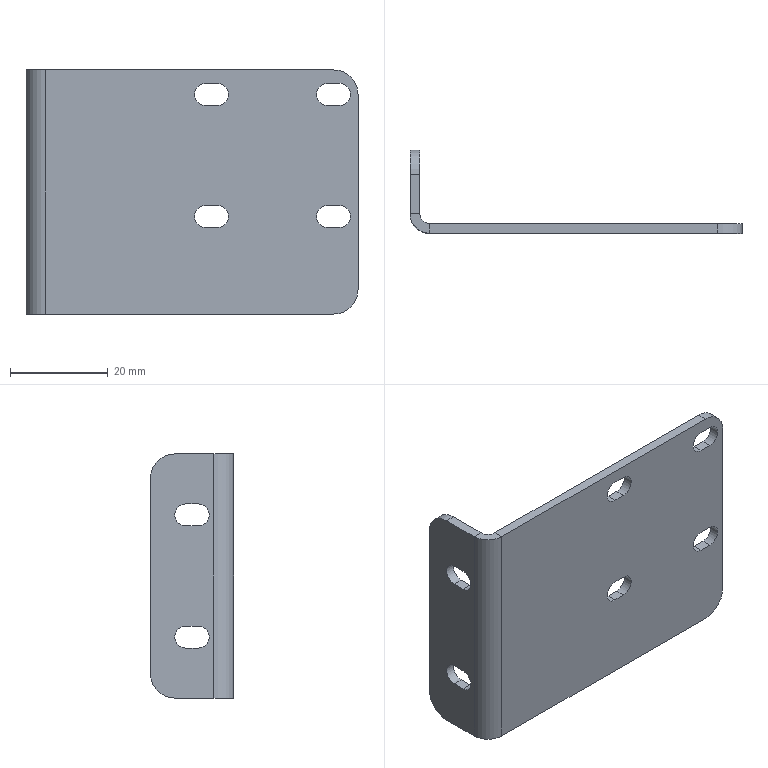Part | SolidWorks | features HoleWzd 2, Fillet 1, FlatPattern 1, SMBaseFlange 1, SheetMetal 1 | 1 solid | 42 faces | box 68 x 17 x 50 mm | volume 7802 mm3 | plane 24 | cylinder 18 | commonest cylinder face diameters 4.5 x12 10 x4 4 x1 8 x1
STEP:
#1=CARTESIAN_POINT('',(2.,-9.75,39.75));
#2=VERTEX_POINT('',#1);
#3=CARTESIAN_POINT('',(2.,-9.75,35.25));
#4=VERTEX_POINT('',#3);
#5=CARTESIAN_POINT('',(2.,-9.75,37.5));
#6=DIRECTION('',(1.,0.,0.));
#7=DIRECTION('',(0.,0.,-1.));
#8=AXIS2_PLACEMENT_3D('',#5,#6,#7);
#9=CIRCLE('',#8,2.25);
#10=EDGE_CURVE('',#2,#4,#9,.T.);
#11=ORIENTED_EDGE('',*,*,#10,.F.);
#12=CARTESIAN_POINT('',(2.,-7.25,39.75));
#13=VERTEX_POINT('',#12);
#14=CARTESIAN_POINT('',(2.,-9.75,39.75));
#15=DIRECTION('',(0.,1.,0.));
#16=VECTOR('',#15,1000.);
#17=LINE('',#14,#16);
#18=EDGE_CURVE('',#2,#13,#17,.T.);
#19=ORIENTED_EDGE('',*,*,#18,.T.);
#20=CARTESIAN_POINT('',(2.,-7.25,35.25));
#21=VERTEX_POINT('',#20);
#22=CARTESIAN_POINT('',(2.,-7.25,37.5));
#23=DIRECTION('',(1.,0.,0.));
#24=DIRECTION('',(0.,0.,-1.));
#25=AXIS2_PLACEMENT_3D('',#22,#23,#24);
#26=CIRCLE('',#25,2.25);
#27=EDGE_CURVE('',#21,#13,#26,.T.);
#28=ORIENTED_EDGE('',*,*,#27,.F.);
#29=CARTESIAN_POINT('',(2.,-9.75,35.25));
#30=DIRECTION('',(0.,1.,0.));
#31=VECTOR('',#30,1000.);
#32=LINE('',#29,#31);
#33=EDGE_CURVE('',#4,#21,#32,.T.);
#34=ORIENTED_EDGE('',*,*,#33,.F.);
#35=EDGE_LOOP('',(#11,#19,#28,#34));
#36=FACE_BOUND('',#35,.T.);
#37=CARTESIAN_POINT('',(2.,0.,45.));
#38=VERTEX_POINT('',#37);
#39=CARTESIAN_POINT('',(2.,0.,5.));
#40=VERTEX_POINT('',#39);
#41=CARTESIAN_POINT('',(2.,0.,50.));
#42=DIRECTION('',(0.,0.,-1.));
#43=VECTOR('',#42,1000.);
#44=LINE('',#41,#43);
#45=EDGE_CURVE('',#38,#40,#44,.T.);
#46=ORIENTED_EDGE('',*,*,#45,.F.);
#47=CARTESIAN_POINT('',(2.,-5.,50.));
#48=VERTEX_POINT('',#47);
#49=CARTESIAN_POINT('',(2.,-5.,45.));
#50=DIRECTION('',(1.,0.,0.));
#51=DIRECTION('',(0.,1.,0.));
#52=AXIS2_PLACEMENT_3D('',#49,#50,#51);
#53=CIRCLE('',#52,5.);
#54=EDGE_CURVE('',#38,#48,#53,.T.);
#55=ORIENTED_EDGE('',*,*,#54,.T.);
#56=CARTESIAN_POINT('',(2.,-13.,50.));
#57=VERTEX_POINT('',#56);
#58=CARTESIAN_POINT('',(2.,0.,50.));
#59=DIRECTION('',(0.,-1.,0.));
#60=VECTOR('',#59,1000.);
#61=LINE('',#58,#60);
#62=EDGE_CURVE('',#48,#57,#61,.T.);
#63=ORIENTED_EDGE('',*,*,#62,.T.);
#64=CARTESIAN_POINT('',(2.,-13.,0.));
#65=VERTEX_POINT('',#64);
#66=CARTESIAN_POINT('',(2.,-13.,50.));
#67=DIRECTION('',(0.,0.,-1.));
#68=VECTOR('',#67,1000.);
#69=LINE('',#66,#68);
#70=EDGE_CURVE('',#57,#65,#69,.T.);
#71=ORIENTED_EDGE('',*,*,#70,.T.);
#72=CARTESIAN_POINT('',(2.,-5.,0.));
#73=VERTEX_POINT('',#72);
#74=CARTESIAN_POINT('',(2.,0.,0.));
#75=DIRECTION('',(0.,-1.,0.));
#76=VECTOR('',#75,1000.);
#77=LINE('',#74,#76);
#78=EDGE_CURVE('',#73,#65,#77,.T.);
#79=ORIENTED_EDGE('',*,*,#78,.F.);
#80=CARTESIAN_POINT('',(2.,-5.,5.));
#81=DIRECTION('',(1.,0.,0.));
#82=DIRECTION('',(0.,1.,0.));
#83=AXIS2_PLACEMENT_3D('',#80,#81,#82);
#84=CIRCLE('',#83,5.);
#85=EDGE_CURVE('',#73,#40,#84,.T.);
#86=ORIENTED_EDGE('',*,*,#85,.T.);
#87=EDGE_LOOP('',(#46,#55,#63,#71,#79,#86));
#88=FACE_OUTER_BOUND('',#87,.T.);
#89=CARTESIAN_POINT('',(2.,-9.75,14.75));
#90=VERTEX_POINT('',#89);
#91=CARTESIAN_POINT('',(2.,-9.75,10.25));
#92=VERTEX_POINT('',#91);
#93=CARTESIAN_POINT('',(2.,-9.75,12.5));
#94=DIRECTION('',(1.,0.,0.));
#95=DIRECTION('',(0.,0.,-1.));
#96=AXIS2_PLACEMENT_3D('',#93,#94,#95);
#97=CIRCLE('',#96,2.25);
#98=EDGE_CURVE('',#90,#92,#97,.T.);
#99=ORIENTED_EDGE('',*,*,#98,.F.);
#100=CARTESIAN_POINT('',(2.,-7.25,14.75));
#101=VERTEX_POINT('',#100);
#102=CARTESIAN_POINT('',(2.,-9.75,14.75));
#103=DIRECTION('',(0.,1.,0.));
#104=VECTOR('',#103,1000.);
#105=LINE('',#102,#104);
#106=EDGE_CURVE('',#90,#101,#105,.T.);
#107=ORIENTED_EDGE('',*,*,#106,.T.);
#108=CARTESIAN_POINT('',(2.,-7.25,10.25));
#109=VERTEX_POINT('',#108);
#110=CARTESIAN_POINT('',(2.,-7.25,12.5));
#111=DIRECTION('',(1.,0.,0.));
#112=DIRECTION('',(0.,0.,-1.));
#113=AXIS2_PLACEMENT_3D('',#110,#111,#112);
#114=CIRCLE('',#113,2.25);
#115=EDGE_CURVE('',#109,#101,#114,.T.);
#116=ORIENTED_EDGE('',*,*,#115,.F.);
#117=CARTESIAN_POINT('',(2.,-9.75,10.25));
#118=DIRECTION('',(0.,1.,0.));
#119=VECTOR('',#118,1000.);
#120=LINE('',#117,#119);
#121=EDGE_CURVE('',#92,#109,#120,.T.);
#122=ORIENTED_EDGE('',*,*,#121,.F.);
#123=EDGE_LOOP('',(#99,#107,#116,#122));
#124=FACE_BOUND('',#123,.T.);
#125=CARTESIAN_POINT('',(2.,0.,50.));
#126=DIRECTION('',(1.,0.,0.));
#127=DIRECTION('',(0.,1.,0.));
#128=AXIS2_PLACEMENT_3D('',#125,#126,#127);
#129=PLANE('',#128);
#130=ADVANCED_FACE('',(#36,#88,#124),#129,.T.);
#131=CARTESIAN_POINT('',(61.75,-15.,47.25));
#132=VERTEX_POINT('',#131);
#133=CARTESIAN_POINT('',(64.25,-15.,47.25));
#134=VERTEX_POINT('',#133);
#135=CARTESIAN_POINT('',(61.75,-15.,47.25));
#136=DIRECTION('',(1.,0.,0.));
#137=VECTOR('',#136,1000.);
#138=LINE('',#135,#137);
#139=EDGE_CURVE('',#132,#134,#138,.T.);
#140=ORIENTED_EDGE('',*,*,#139,.F.);
#141=CARTESIAN_POINT('',(61.75,-15.,42.75));
#142=VERTEX_POINT('',#141);
#143=CARTESIAN_POINT('',(61.75,-15.,45.));
#144=DIRECTION('',(0.,1.,0.));
#145=DIRECTION('',(0.,0.,1.));
#146=AXIS2_PLACEMENT_3D('',#143,#144,#145);
#147=CIRCLE('',#146,2.25);
#148=EDGE_CURVE('',#142,#132,#147,.T.);
#149=ORIENTED_EDGE('',*,*,#148,.F.);
#150=CARTESIAN_POINT('',(64.25,-15.,42.75));
#151=VERTEX_POINT('',#150);
#152=CARTESIAN_POINT('',(61.75,-15.,42.75));
#153=DIRECTION('',(1.,0.,0.));
#154=VECTOR('',#153,1000.);
#155=LINE('',#152,#154);
#156=EDGE_CURVE('',#142,#151,#155,.T.);
#157=ORIENTED_EDGE('',*,*,#156,.T.);
#158=CARTESIAN_POINT('',(64.25,-15.,45.));
#159=DIRECTION('',(0.,1.,0.));
#160=DIRECTION('',(0.,0.,1.));
#161=AXIS2_PLACEMENT_3D('',#158,#159,#160);
#162=CIRCLE('',#161,2.25);
#163=EDGE_CURVE('',#134,#151,#162,.T.);
#164=ORIENTED_EDGE('',*,*,#163,.F.);
#165=EDGE_LOOP('',(#140,#149,#157,#164));
#166=FACE_BOUND('',#165,.T.);
#167=CARTESIAN_POINT('',(36.75,-15.,42.75));
#168=VERTEX_POINT('',#167);
#169=CARTESIAN_POINT('',(39.25,-15.,42.75));
#170=VERTEX_POINT('',#169);
#171=CARTESIAN_POINT('',(36.75,-15.,42.75));
#172=DIRECTION('',(1.,0.,0.));
#173=VECTOR('',#172,1000.);
#174=LINE('',#171,#173);
#175=EDGE_CURVE('',#168,#170,#174,.T.);
#176=ORIENTED_EDGE('',*,*,#175,.T.);
#177=CARTESIAN_POINT('',(39.25,-15.,47.25));
#178=VERTEX_POINT('',#177);
#179=CARTESIAN_POINT('',(39.25,-15.,45.));
#180=DIRECTION('',(0.,1.,0.));
#181=DIRECTION('',(0.,0.,1.));
#182=AXIS2_PLACEMENT_3D('',#179,#180,#181);
#183=CIRCLE('',#182,2.25);
#184=EDGE_CURVE('',#178,#170,#183,.T.);
#185=ORIENTED_EDGE('',*,*,#184,.F.);
#186=CARTESIAN_POINT('',(36.75,-15.,47.25));
#187=VERTEX_POINT('',#186);
#188=CARTESIAN_POINT('',(36.75,-15.,47.25));
#189=DIRECTION('',(1.,0.,0.));
#190=VECTOR('',#189,1000.);
#191=LINE('',#188,#190);
#192=EDGE_CURVE('',#187,#178,#191,.T.);
#193=ORIENTED_EDGE('',*,*,#192,.F.);
#194=CARTESIAN_POINT('',(36.75,-15.,45.));
#195=DIRECTION('',(0.,1.,0.));
#196=DIRECTION('',(0.,0.,1.));
#197=AXIS2_PLACEMENT_3D('',#194,#195,#196);
#198=CIRCLE('',#197,2.25);
#199=EDGE_CURVE('',#168,#187,#198,.T.);
#200=ORIENTED_EDGE('',*,*,#199,.F.);
#201=EDGE_LOOP('',(#176,#185,#193,#200));
#202=FACE_BOUND('',#201,.T.);
#203=CARTESIAN_POINT('',(36.75,-15.,22.25));
#204=VERTEX_POINT('',#203);
#205=CARTESIAN_POINT('',(39.25,-15.,22.25));
#206=VERTEX_POINT('',#205);
#207=CARTESIAN_POINT('',(36.75,-15.,22.25));
#208=DIRECTION('',(1.,0.,0.));
#209=VECTOR('',#208,1000.);
#210=LINE('',#207,#209);
#211=EDGE_CURVE('',#204,#206,#210,.T.);
#212=ORIENTED_EDGE('',*,*,#211,.F.);
#213=CARTESIAN_POINT('',(36.75,-15.,17.75));
#214=VERTEX_POINT('',#213);
#215=CARTESIAN_POINT('',(36.75,-15.,20.));
#216=DIRECTION('',(0.,1.,0.));
#217=DIRECTION('',(0.,0.,1.));
#218=AXIS2_PLACEMENT_3D('',#215,#216,#217);
#219=CIRCLE('',#218,2.25);
#220=EDGE_CURVE('',#214,#204,#219,.T.);
#221=ORIENTED_EDGE('',*,*,#220,.F.);
#222=CARTESIAN_POINT('',(39.25,-15.,17.75));
#223=VERTEX_POINT('',#222);
#224=CARTESIAN_POINT('',(36.75,-15.,17.75));
#225=DIRECTION('',(1.,0.,0.));
#226=VECTOR('',#225,1000.);
#227=LINE('',#224,#226);
#228=EDGE_CURVE('',#214,#223,#227,.T.);
#229=ORIENTED_EDGE('',*,*,#228,.T.);
#230=CARTESIAN_POINT('',(39.25,-15.,20.));
#231=DIRECTION('',(0.,1.,0.));
#232=DIRECTION('',(0.,0.,1.));
#233=AXIS2_PLACEMENT_3D('',#230,#231,#232);
#234=CIRCLE('',#233,2.25);
#235=EDGE_CURVE('',#206,#223,#234,.T.);
#236=ORIENTED_EDGE('',*,*,#235,.F.);
#237=EDGE_LOOP('',(#212,#221,#229,#236));
#238=FACE_BOUND('',#237,.T.);
#239=CARTESIAN_POINT('',(4.,-15.,50.));
#240=VERTEX_POINT('',#239);
#241=CARTESIAN_POINT('',(63.,-15.,50.));
#242=VERTEX_POINT('',#241);
#243=CARTESIAN_POINT('',(0.,-15.,50.));
#244=DIRECTION('',(1.,0.,0.));
#245=VECTOR('',#244,1000.);
#246=LINE('',#243,#245);
#247=EDGE_CURVE('',#240,#242,#246,.T.);
#248=ORIENTED_EDGE('',*,*,#247,.T.);
#249=CARTESIAN_POINT('',(68.,-15.,45.));
#250=VERTEX_POINT('',#249);
#251=CARTESIAN_POINT('',(63.,-15.,45.));
#252=DIRECTION('',(0.,1.,0.));
#253=DIRECTION('',(0.,0.,1.));
#254=AXIS2_PLACEMENT_3D('',#251,#252,#253);
#255=CIRCLE('',#254,5.);
#256=EDGE_CURVE('',#242,#250,#255,.T.);
#257=ORIENTED_EDGE('',*,*,#256,.T.);
#258=CARTESIAN_POINT('',(68.,-15.,5.));
#259=VERTEX_POINT('',#258);
#260=CARTESIAN_POINT('',(68.,-15.,50.));
#261=DIRECTION('',(0.,0.,-1.));
#262=VECTOR('',#261,1000.);
#263=LINE('',#260,#262);
#264=EDGE_CURVE('',#250,#259,#263,.T.);
#265=ORIENTED_EDGE('',*,*,#264,.T.);
#266=CARTESIAN_POINT('',(63.,-15.,0.));
#267=VERTEX_POINT('',#266);
#268=CARTESIAN_POINT('',(63.,-15.,5.));
#269=DIRECTION('',(0.,1.,0.));
#270=DIRECTION('',(0.,0.,1.));
#271=AXIS2_PLACEMENT_3D('',#268,#269,#270);
#272=CIRCLE('',#271,5.);
#273=EDGE_CURVE('',#259,#267,#272,.T.);
#274=ORIENTED_EDGE('',*,*,#273,.T.);
#275=CARTESIAN_POINT('',(4.,-15.,0.));
#276=VERTEX_POINT('',#275);
#277=CARTESIAN_POINT('',(0.,-15.,0.));
#278=DIRECTION('',(1.,0.,0.));
#279=VECTOR('',#278,1000.);
#280=LINE('',#277,#279);
#281=EDGE_CURVE('',#276,#267,#280,.T.);
#282=ORIENTED_EDGE('',*,*,#281,.F.);
#283=CARTESIAN_POINT('',(4.,-15.,50.));
#284=DIRECTION('',(0.,0.,-1.));
#285=VECTOR('',#284,1000.);
#286=LINE('',#283,#285);
#287=EDGE_CURVE('',#240,#276,#286,.T.);
#288=ORIENTED_EDGE('',*,*,#287,.F.);
#289=EDGE_LOOP('',(#248,#257,#265,#274,#282,#288));
#290=FACE_OUTER_BOUND('',#289,.T.);
#291=CARTESIAN_POINT('',(61.75,-15.,17.75));
#292=VERTEX_POINT('',#291);
#293=CARTESIAN_POINT('',(61.75,-15.,22.25));
#294=VERTEX_POINT('',#293);
#295=CARTESIAN_POINT('',(61.75,-15.,20.));
#296=DIRECTION('',(0.,1.,0.));
#297=DIRECTION('',(0.,0.,1.));
#298=AXIS2_PLACEMENT_3D('',#295,#296,#297);
#299=CIRCLE('',#298,2.25);
#300=EDGE_CURVE('',#292,#294,#299,.T.);
#301=ORIENTED_EDGE('',*,*,#300,.F.);
#302=CARTESIAN_POINT('',(64.25,-15.,17.75));
#303=VERTEX_POINT('',#302);
#304=CARTESIAN_POINT('',(61.75,-15.,17.75));
#305=DIRECTION('',(1.,0.,0.));
#306=VECTOR('',#305,1000.);
#307=LINE('',#304,#306);
#308=EDGE_CURVE('',#292,#303,#307,.T.);
#309=ORIENTED_EDGE('',*,*,#308,.T.);
#310=CARTESIAN_POINT('',(64.25,-15.,22.25));
#311=VERTEX_POINT('',#310);
#312=CARTESIAN_POINT('',(64.25,-15.,20.));
#313=DIRECTION('',(0.,1.,0.));
#314=DIRECTION('',(0.,0.,1.));
#315=AXIS2_PLACEMENT_3D('',#312,#313,#314);
#316=CIRCLE('',#315,2.25);
#317=EDGE_CURVE('',#311,#303,#316,.T.);
#318=ORIENTED_EDGE('',*,*,#317,.F.);
#319=CARTESIAN_POINT('',(61.75,-15.,22.25));
#320=DIRECTION('',(1.,0.,0.));
#321=VECTOR('',#320,1000.);
#322=LINE('',#319,#321);
#323=EDGE_CURVE('',#294,#311,#322,.T.);
#324=ORIENTED_EDGE('',*,*,#323,.F.);
#325=EDGE_LOOP('',(#301,#309,#318,#324));
#326=FACE_BOUND('',#325,.T.);
#327=CARTESIAN_POINT('',(0.,-15.,50.));
#328=DIRECTION('',(0.,1.,0.));
#329=DIRECTION('',(0.,0.,1.));
#330=AXIS2_PLACEMENT_3D('',#327,#328,#329);
#331=PLANE('',#330);
#332=ADVANCED_FACE('',(#166,#202,#238,#290,#326),#331,.T.);
#333=CARTESIAN_POINT('',(0.,-13.,50.));
#334=VERTEX_POINT('',#333);
#335=CARTESIAN_POINT('',(0.,-13.,50.));
#336=DIRECTION('',(1.,0.,0.));
#337=VECTOR('',#336,1000.);
#338=LINE('',#335,#337);
#339=EDGE_CURVE('',#334,#57,#338,.T.);
#340=ORIENTED_EDGE('',*,*,#339,.F.);
#341=CARTESIAN_POINT('',(4.,-17.,50.));
#342=VERTEX_POINT('',#341);
#343=CARTESIAN_POINT('',(4.,-13.,50.));
#344=DIRECTION('',(0.,0.,1.));
#345=DIRECTION('',(-1.,0.,0.));
#346=AXIS2_PLACEMENT_3D('',#343,#344,#345);
#347=CIRCLE('',#346,4.);
#348=EDGE_CURVE('',#334,#342,#347,.T.);
#349=ORIENTED_EDGE('',*,*,#348,.T.);
#350=CARTESIAN_POINT('',(4.,-15.,50.));
#351=DIRECTION('',(0.,-1.,0.));
#352=VECTOR('',#351,1000.);
#353=LINE('',#350,#352);
#354=EDGE_CURVE('',#240,#342,#353,.T.);
#355=ORIENTED_EDGE('',*,*,#354,.F.);
#356=CARTESIAN_POINT('',(4.,-13.,50.));
#357=DIRECTION('',(0.,0.,1.));
#358=DIRECTION('',(1.,0.,0.));
#359=AXIS2_PLACEMENT_3D('',#356,#357,#358);
#360=CIRCLE('',#359,2.);
#361=EDGE_CURVE('',#57,#240,#360,.T.);
#362=ORIENTED_EDGE('',*,*,#361,.F.);
#363=EDGE_LOOP('',(#340,#349,#355,#362));
#364=FACE_OUTER_BOUND('',#363,.T.);
#365=CARTESIAN_POINT('',(0.,-13.,50.));
#366=DIRECTION('',(0.,0.,1.));
#367=DIRECTION('',(1.,0.,0.));
#368=AXIS2_PLACEMENT_3D('',#365,#366,#367);
#369=PLANE('',#368);
#370=ADVANCED_FACE('',(#364),#369,.T.);
#371=ORIENTED_EDGE('',*,*,#62,.F.);
#372=CARTESIAN_POINT('',(0.,-5.,50.));
#373=VERTEX_POINT('',#372);
#374=CARTESIAN_POINT('',(4.,-5.,50.));
#375=DIRECTION('',(-1.,0.,0.));
#376=VECTOR('',#375,1000.);
#377=LINE('',#374,#376);
#378=EDGE_CURVE('',#48,#373,#377,.T.);
#379=ORIENTED_EDGE('',*,*,#378,.T.);
#380=CARTESIAN_POINT('',(0.,0.,50.));
#381=DIRECTION('',(0.,-1.,0.));
#382=VECTOR('',#381,1000.);
#383=LINE('',#380,#382);
#384=EDGE_CURVE('',#373,#334,#383,.T.);
#385=ORIENTED_EDGE('',*,*,#384,.T.);
#386=ORIENTED_EDGE('',*,*,#339,.T.);
#387=EDGE_LOOP('',(#371,#379,#385,#386));
#388=FACE_OUTER_BOUND('',#387,.T.);
#389=CARTESIAN_POINT('',(4.,-15.,50.));
#390=DIRECTION('',(0.,0.,1.));
#391=DIRECTION('',(1.,0.,0.));
#392=AXIS2_PLACEMENT_3D('',#389,#390,#391);
#393=PLANE('',#392);
#394=ADVANCED_FACE('',(#388),#393,.T.);
#395=CARTESIAN_POINT('',(4.,-17.,0.));
#396=VERTEX_POINT('',#395);
#397=CARTESIAN_POINT('',(4.,-17.,0.));
#398=DIRECTION('',(0.,1.,0.));
#399=VECTOR('',#398,1000.);
#400=LINE('',#397,#399);
#401=EDGE_CURVE('',#396,#276,#400,.T.);
#402=ORIENTED_EDGE('',*,*,#401,.F.);
#403=CARTESIAN_POINT('',(0.,-13.,0.));
#404=VERTEX_POINT('',#403);
#405=CARTESIAN_POINT('',(4.,-13.,0.));
#406=DIRECTION('',(0.,0.,1.));
#407=DIRECTION('',(-1.,0.,0.));
#408=AXIS2_PLACEMENT_3D('',#405,#406,#407);
#409=CIRCLE('',#408,4.);
#410=EDGE_CURVE('',#404,#396,#409,.T.);
#411=ORIENTED_EDGE('',*,*,#410,.F.);
#412=CARTESIAN_POINT('',(2.,-13.,0.));
#413=DIRECTION('',(-1.,0.,0.));
#414=VECTOR('',#413,1000.);
#415=LINE('',#412,#414);
#416=EDGE_CURVE('',#65,#404,#415,.T.);
#417=ORIENTED_EDGE('',*,*,#416,.F.);
#418=CARTESIAN_POINT('',(4.,-13.,0.));
#419=DIRECTION('',(0.,0.,1.));
#420=DIRECTION('',(1.,0.,0.));
#421=AXIS2_PLACEMENT_3D('',#418,#419,#420);
#422=CIRCLE('',#421,2.);
#423=EDGE_CURVE('',#65,#276,#422,.T.);
#424=ORIENTED_EDGE('',*,*,#423,.T.);
#425=EDGE_LOOP('',(#402,#411,#417,#424));
#426=FACE_OUTER_BOUND('',#425,.T.);
#427=CARTESIAN_POINT('',(4.,-17.,0.));
#428=DIRECTION('',(0.,0.,-1.));
#429=DIRECTION('',(-1.,0.,0.));
#430=AXIS2_PLACEMENT_3D('',#427,#428,#429);
#431=PLANE('',#430);
#432=ADVANCED_FACE('',(#426),#431,.T.);
#433=ORIENTED_EDGE('',*,*,#281,.T.);
#434=CARTESIAN_POINT('',(63.,-17.,0.));
#435=VERTEX_POINT('',#434);
#436=CARTESIAN_POINT('',(63.,-13.,0.));
#437=DIRECTION('',(0.,-1.,0.));
#438=VECTOR('',#437,1000.);
#439=LINE('',#436,#438);
#440=EDGE_CURVE('',#267,#435,#439,.T.);
#441=ORIENTED_EDGE('',*,*,#440,.T.);
#442=CARTESIAN_POINT('',(0.,-17.,0.));
#443=DIRECTION('',(1.,0.,0.));
#444=VECTOR('',#443,1000.);
#445=LINE('',#442,#444);
#446=EDGE_CURVE('',#396,#435,#445,.T.);
#447=ORIENTED_EDGE('',*,*,#446,.F.);
#448=ORIENTED_EDGE('',*,*,#401,.T.);
#449=EDGE_LOOP('',(#433,#441,#447,#448));
#450=FACE_OUTER_BOUND('',#449,.T.);
#451=CARTESIAN_POINT('',(2.,-13.,0.));
#452=DIRECTION('',(0.,0.,-1.));
#453=DIRECTION('',(-1.,0.,0.));
#454=AXIS2_PLACEMENT_3D('',#451,#452,#453);
#455=PLANE('',#454);
#456=ADVANCED_FACE('',(#450),#455,.T.);
#457=CARTESIAN_POINT('',(61.75,-17.,47.25));
#458=VERTEX_POINT('',#457);
#459=CARTESIAN_POINT('',(64.25,-17.,47.25));
#460=VERTEX_POINT('',#459);
#461=CARTESIAN_POINT('',(61.75,-17.,47.25));
#462=DIRECTION('',(1.,0.,0.));
#463=VECTOR('',#462,1000.);
#464=LINE('',#461,#463);
#465=EDGE_CURVE('',#458,#460,#464,.T.);
#466=ORIENTED_EDGE('',*,*,#465,.T.);
#467=CARTESIAN_POINT('',(64.25,-17.,42.75));
#468=VERTEX_POINT('',#467);
#469=CARTESIAN_POINT('',(64.25,-17.,45.));
#470=DIRECTION('',(0.,1.,0.));
#471=DIRECTION('',(0.,0.,1.));
#472=AXIS2_PLACEMENT_3D('',#469,#470,#471);
#473=CIRCLE('',#472,2.25);
#474=EDGE_CURVE('',#460,#468,#473,.T.);
#475=ORIENTED_EDGE('',*,*,#474,.T.);
#476=CARTESIAN_POINT('',(61.75,-17.,42.75));
#477=VERTEX_POINT('',#476);
#478=CARTESIAN_POINT('',(61.75,-17.,42.75));
#479=DIRECTION('',(1.,0.,0.));
#480=VECTOR('',#479,1000.);
#481=LINE('',#478,#480);
#482=EDGE_CURVE('',#477,#468,#481,.T.);
#483=ORIENTED_EDGE('',*,*,#482,.F.);
#484=CARTESIAN_POINT('',(61.75,-17.,45.));
#485=DIRECTION('',(0.,1.,0.));
#486=DIRECTION('',(0.,0.,1.));
#487=AXIS2_PLACEMENT_3D('',#484,#485,#486);
#488=CIRCLE('',#487,2.25);
#489=EDGE_CURVE('',#477,#458,#488,.T.);
#490=ORIENTED_EDGE('',*,*,#489,.T.);
#491=EDGE_LOOP('',(#466,#475,#483,#490));
#492=FACE_BOUND('',#491,.T.);
#493=CARTESIAN_POINT('',(36.75,-17.,47.25));
#494=VERTEX_POINT('',#493);
#495=CARTESIAN_POINT('',(39.25,-17.,47.25));
#496=VERTEX_POINT('',#495);
#497=CARTESIAN_POINT('',(36.75,-17.,47.25));
#498=DIRECTION('',(1.,0.,0.));
#499=VECTOR('',#498,1000.);
#500=LINE('',#497,#499);
#501=EDGE_CURVE('',#494,#496,#500,.T.);
#502=ORIENTED_EDGE('',*,*,#501,.T.);
#503=CARTESIAN_POINT('',(39.25,-17.,42.75));
#504=VERTEX_POINT('',#503);
#505=CARTESIAN_POINT('',(39.25,-17.,45.));
#506=DIRECTION('',(0.,1.,0.));
#507=DIRECTION('',(0.,0.,1.));
#508=AXIS2_PLACEMENT_3D('',#505,#506,#507);
#509=CIRCLE('',#508,2.25);
#510=EDGE_CURVE('',#496,#504,#509,.T.);
#511=ORIENTED_EDGE('',*,*,#510,.T.);
#512=CARTESIAN_POINT('',(36.75,-17.,42.75));
#513=VERTEX_POINT('',#512);
#514=CARTESIAN_POINT('',(36.75,-17.,42.75));
#515=DIRECTION('',(1.,0.,0.));
#516=VECTOR('',#515,1000.);
#517=LINE('',#514,#516);
#518=EDGE_CURVE('',#513,#504,#517,.T.);
#519=ORIENTED_EDGE('',*,*,#518,.F.);
#520=CARTESIAN_POINT('',(36.75,-17.,45.));
#521=DIRECTION('',(0.,1.,0.));
#522=DIRECTION('',(0.,0.,1.));
#523=AXIS2_PLACEMENT_3D('',#520,#521,#522);
#524=CIRCLE('',#523,2.25);
#525=EDGE_CURVE('',#513,#494,#524,.T.);
#526=ORIENTED_EDGE('',*,*,#525,.T.);
#527=EDGE_LOOP('',(#502,#511,#519,#526));
#528=FACE_BOUND('',#527,.T.);
#529=CARTESIAN_POINT('',(61.75,-17.,22.25));
#530=VERTEX_POINT('',#529);
#531=CARTESIAN_POINT('',(64.25,-17.,22.25));
#532=VERTEX_POINT('',#531);
#533=CARTESIAN_POINT('',(61.75,-17.,22.25));
#534=DIRECTION('',(1.,0.,0.));
#535=VECTOR('',#534,1000.);
#536=LINE('',#533,#535);
#537=EDGE_CURVE('',#530,#532,#536,.T.);
#538=ORIENTED_EDGE('',*,*,#537,.T.);
#539=CARTESIAN_POINT('',(64.25,-17.,17.75));
#540=VERTEX_POINT('',#539);
#541=CARTESIAN_POINT('',(64.25,-17.,20.));
#542=DIRECTION('',(0.,1.,0.));
#543=DIRECTION('',(0.,0.,1.));
#544=AXIS2_PLACEMENT_3D('',#541,#542,#543);
#545=CIRCLE('',#544,2.25);
#546=EDGE_CURVE('',#532,#540,#545,.T.);
#547=ORIENTED_EDGE('',*,*,#546,.T.);
#548=CARTESIAN_POINT('',(61.75,-17.,17.75));
#549=VERTEX_POINT('',#548);
#550=CARTESIAN_POINT('',(61.75,-17.,17.75));
#551=DIRECTION('',(1.,0.,0.));
#552=VECTOR('',#551,1000.);
#553=LINE('',#550,#552);
#554=EDGE_CURVE('',#549,#540,#553,.T.);
#555=ORIENTED_EDGE('',*,*,#554,.F.);
#556=CARTESIAN_POINT('',(61.75,-17.,20.));
#557=DIRECTION('',(0.,1.,0.));
#558=DIRECTION('',(0.,0.,1.));
#559=AXIS2_PLACEMENT_3D('',#556,#557,#558);
#560=CIRCLE('',#559,2.25);
#561=EDGE_CURVE('',#549,#530,#560,.T.);
#562=ORIENTED_EDGE('',*,*,#561,.T.);
#563=EDGE_LOOP('',(#538,#547,#555,#562));
#564=FACE_BOUND('',#563,.T.);
#565=CARTESIAN_POINT('',(36.75,-17.,17.75));
#566=VERTEX_POINT('',#565);
#567=CARTESIAN_POINT('',(36.75,-17.,22.25));
#568=VERTEX_POINT('',#567);
#569=CARTESIAN_POINT('',(36.75,-17.,20.));
#570=DIRECTION('',(0.,1.,0.));
#571=DIRECTION('',(0.,0.,1.));
#572=AXIS2_PLACEMENT_3D('',#569,#570,#571);
#573=CIRCLE('',#572,2.25);
#574=EDGE_CURVE('',#566,#568,#573,.T.);
#575=ORIENTED_EDGE('',*,*,#574,.T.);
#576=CARTESIAN_POINT('',(39.25,-17.,22.25));
#577=VERTEX_POINT('',#576);
#578=CARTESIAN_POINT('',(36.75,-17.,22.25));
#579=DIRECTION('',(1.,0.,0.));
#580=VECTOR('',#579,1000.);
#581=LINE('',#578,#580);
#582=EDGE_CURVE('',#568,#577,#581,.T.);
#583=ORIENTED_EDGE('',*,*,#582,.T.);
#584=CARTESIAN_POINT('',(39.25,-17.,17.75));
#585=VERTEX_POINT('',#584);
#586=CARTESIAN_POINT('',(39.25,-17.,20.));
#587=DIRECTION('',(0.,1.,0.));
#588=DIRECTION('',(0.,0.,1.));
#589=AXIS2_PLACEMENT_3D('',#586,#587,#588);
#590=CIRCLE('',#589,2.25);
#591=EDGE_CURVE('',#577,#585,#590,.T.);
#592=ORIENTED_EDGE('',*,*,#591,.T.);
#593=CARTESIAN_POINT('',(36.75,-17.,17.75));
#594=DIRECTION('',(1.,0.,0.));
#595=VECTOR('',#594,1000.);
#596=LINE('',#593,#595);
#597=EDGE_CURVE('',#566,#585,#596,.T.);
#598=ORIENTED_EDGE('',*,*,#597,.F.);
#599=EDGE_LOOP('',(#575,#583,#592,#598));
#600=FACE_BOUND('',#599,.T.);
#601=CARTESIAN_POINT('',(68.,-17.,45.));
#602=VERTEX_POINT('',#601);
#603=CARTESIAN_POINT('',(68.,-17.,5.));
#604=VERTEX_POINT('',#603);
#605=CARTESIAN_POINT('',(68.,-17.,50.));
#606=DIRECTION('',(0.,0.,-1.));
#607=VECTOR('',#606,1000.);
#608=LINE('',#605,#607);
#609=EDGE_CURVE('',#602,#604,#608,.T.);
#610=ORIENTED_EDGE('',*,*,#609,.F.);
#611=CARTESIAN_POINT('',(63.,-17.,50.));
#612=VERTEX_POINT('',#611);
#613=CARTESIAN_POINT('',(63.,-17.,45.));
#614=DIRECTION('',(0.,-1.,0.));
#615=DIRECTION('',(0.,0.,1.));
#616=AXIS2_PLACEMENT_3D('',#613,#614,#615);
#617=CIRCLE('',#616,5.);
#618=EDGE_CURVE('',#602,#612,#617,.T.);
#619=ORIENTED_EDGE('',*,*,#618,.T.);
#620=CARTESIAN_POINT('',(0.,-17.,50.));
#621=DIRECTION('',(1.,0.,0.));
#622=VECTOR('',#621,1000.);
#623=LINE('',#620,#622);
#624=EDGE_CURVE('',#342,#612,#623,.T.);
#625=ORIENTED_EDGE('',*,*,#624,.F.);
#626=CARTESIAN_POINT('',(4.,-17.,50.));
#627=DIRECTION('',(0.,0.,-1.));
#628=VECTOR('',#627,1000.);
#629=LINE('',#626,#628);
#630=EDGE_CURVE('',#342,#396,#629,.T.);
#631=ORIENTED_EDGE('',*,*,#630,.T.);
#632=ORIENTED_EDGE('',*,*,#446,.T.);
#633=CARTESIAN_POINT('',(63.,-17.,5.));
#634=DIRECTION('',(0.,-1.,0.));
#635=DIRECTION('',(0.,0.,1.));
#636=AXIS2_PLACEMENT_3D('',#633,#634,#635);
#637=CIRCLE('',#636,5.);
#638=EDGE_CURVE('',#435,#604,#637,.T.);
#639=ORIENTED_EDGE('',*,*,#638,.T.);
#640=EDGE_LOOP('',(#610,#619,#625,#631,#632,#639));
#641=FACE_OUTER_BOUND('',#640,.T.);
#642=CARTESIAN_POINT('',(0.,-17.,50.));
#643=DIRECTION('',(0.,1.,0.));
#644=DIRECTION('',(0.,0.,1.));
#645=AXIS2_PLACEMENT_3D('',#642,#643,#644);
#646=PLANE('',#645);
#647=ADVANCED_FACE('',(#492,#528,#564,#600,#641),#646,.F.);
#648=ORIENTED_EDGE('',*,*,#264,.F.);
#649=CARTESIAN_POINT('',(68.,-15.,45.));
#650=DIRECTION('',(0.,-1.,0.));
#651=VECTOR('',#650,1000.);
#652=LINE('',#649,#651);
#653=EDGE_CURVE('',#250,#602,#652,.T.);
#654=ORIENTED_EDGE('',*,*,#653,.T.);
#655=ORIENTED_EDGE('',*,*,#609,.T.);
#656=CARTESIAN_POINT('',(68.,-15.,5.));
#657=DIRECTION('',(0.,1.,0.));
#658=VECTOR('',#657,1000.);
#659=LINE('',#656,#658);
#660=EDGE_CURVE('',#604,#259,#659,.T.);
#661=ORIENTED_EDGE('',*,*,#660,.T.);
#662=EDGE_LOOP('',(#648,#654,#655,#661));
#663=FACE_OUTER_BOUND('',#662,.T.);
#664=CARTESIAN_POINT('',(68.,-15.,50.));
#665=DIRECTION('',(1.,0.,0.));
#666=DIRECTION('',(0.,0.,-1.));
#667=AXIS2_PLACEMENT_3D('',#664,#665,#666);
#668=PLANE('',#667);
#669=ADVANCED_FACE('',(#663),#668,.T.);
#670=ORIENTED_EDGE('',*,*,#423,.F.);
#671=ORIENTED_EDGE('',*,*,#70,.F.);
#672=ORIENTED_EDGE('',*,*,#361,.T.);
#673=ORIENTED_EDGE('',*,*,#287,.T.);
#674=EDGE_LOOP('',(#670,#671,#672,#673));
#675=FACE_OUTER_BOUND('',#674,.T.);
#676=CARTESIAN_POINT('',(4.,-13.,50.));
#677=DIRECTION('',(0.,0.,-1.));
#678=DIRECTION('',(-1.,0.,0.));
#679=AXIS2_PLACEMENT_3D('',#676,#677,#678);
#680=CYLINDRICAL_SURFACE('',#679,2.);
#681=ADVANCED_FACE('',(#675),#680,.F.);
#682=CARTESIAN_POINT('',(0.,0.,45.));
#683=VERTEX_POINT('',#682);
#684=CARTESIAN_POINT('',(0.,0.,5.));
#685=VERTEX_POINT('',#684);
#686=CARTESIAN_POINT('',(0.,0.,50.));
#687=DIRECTION('',(0.,0.,-1.));
#688=VECTOR('',#687,1000.);
#689=LINE('',#686,#688);
#690=EDGE_CURVE('',#683,#685,#689,.T.);
#691=ORIENTED_EDGE('',*,*,#690,.F.);
#692=CARTESIAN_POINT('',(0.,0.,45.));
#693=DIRECTION('',(1.,0.,0.));
#694=VECTOR('',#693,1000.);
#695=LINE('',#692,#694);
#696=EDGE_CURVE('',#683,#38,#695,.T.);
#697=ORIENTED_EDGE('',*,*,#696,.T.);
#698=ORIENTED_EDGE('',*,*,#45,.T.);
#699=CARTESIAN_POINT('',(0.,0.,5.));
#700=DIRECTION('',(-1.,0.,0.));
#701=VECTOR('',#700,1000.);
#702=LINE('',#699,#701);
#703=EDGE_CURVE('',#40,#685,#702,.T.);
#704=ORIENTED_EDGE('',*,*,#703,.T.);
#705=EDGE_LOOP('',(#691,#697,#698,#704));
#706=FACE_OUTER_BOUND('',#705,.T.);
#707=CARTESIAN_POINT('',(0.,0.,50.));
#708=DIRECTION('',(0.,1.,0.));
#709=DIRECTION('',(-1.,0.,0.));
#710=AXIS2_PLACEMENT_3D('',#707,#708,#709);
#711=PLANE('',#710);
#712=ADVANCED_FACE('',(#706),#711,.T.);
#713=CARTESIAN_POINT('',(0.,-9.75,14.75));
#714=VERTEX_POINT('',#713);
#715=CARTESIAN_POINT('',(0.,-9.75,10.25));
#716=VERTEX_POINT('',#715);
#717=CARTESIAN_POINT('',(0.,-9.75,12.5));
#718=DIRECTION('',(1.,0.,0.));
#719=DIRECTION('',(0.,1.,0.));
#720=AXIS2_PLACEMENT_3D('',#717,#718,#719);
#721=CIRCLE('',#720,2.25);
#722=EDGE_CURVE('',#714,#716,#721,.T.);
#723=ORIENTED_EDGE('',*,*,#722,.T.);
#724=CARTESIAN_POINT('',(0.,-7.25,10.25));
#725=VERTEX_POINT('',#724);
#726=CARTESIAN_POINT('',(0.,0.,10.25));
#727=DIRECTION('',(0.,1.,0.));
#728=VECTOR('',#727,1000.);
#729=LINE('',#726,#728);
#730=EDGE_CURVE('',#716,#725,#729,.T.);
#731=ORIENTED_EDGE('',*,*,#730,.T.);
#732=CARTESIAN_POINT('',(0.,-7.25,14.75));
#733=VERTEX_POINT('',#732);
#734=CARTESIAN_POINT('',(0.,-7.25,12.5));
#735=DIRECTION('',(1.,0.,0.));
#736=DIRECTION('',(0.,1.,0.));
#737=AXIS2_PLACEMENT_3D('',#734,#735,#736);
#738=CIRCLE('',#737,2.25);
#739=EDGE_CURVE('',#725,#733,#738,.T.);
#740=ORIENTED_EDGE('',*,*,#739,.T.);
#741=CARTESIAN_POINT('',(0.,0.,14.75));
#742=DIRECTION('',(0.,-1.,0.));
#743=VECTOR('',#742,1000.);
#744=LINE('',#741,#743);
#745=EDGE_CURVE('',#733,#714,#744,.T.);
#746=ORIENTED_EDGE('',*,*,#745,.T.);
#747=EDGE_LOOP('',(#723,#731,#740,#746));
#748=FACE_BOUND('',#747,.T.);
#749=CARTESIAN_POINT('',(0.,-9.75,35.25));
#750=VERTEX_POINT('',#749);
#751=CARTESIAN_POINT('',(0.,-7.25,35.25));
#752=VERTEX_POINT('',#751);
#753=CARTESIAN_POINT('',(0.,0.,35.25));
#754=DIRECTION('',(0.,1.,0.));
#755=VECTOR('',#754,1000.);
#756=LINE('',#753,#755);
#757=EDGE_CURVE('',#750,#752,#756,.T.);
#758=ORIENTED_EDGE('',*,*,#757,.T.);
#759=CARTESIAN_POINT('',(0.,-7.25,39.75));
#760=VERTEX_POINT('',#759);
#761=CARTESIAN_POINT('',(0.,-7.25,37.5));
#762=DIRECTION('',(1.,0.,0.));
#763=DIRECTION('',(0.,1.,0.));
#764=AXIS2_PLACEMENT_3D('',#761,#762,#763);
#765=CIRCLE('',#764,2.25);
#766=EDGE_CURVE('',#752,#760,#765,.T.);
#767=ORIENTED_EDGE('',*,*,#766,.T.);
#768=CARTESIAN_POINT('',(0.,-9.75,39.75));
#769=VERTEX_POINT('',#768);
#770=CARTESIAN_POINT('',(0.,0.,39.75));
#771=DIRECTION('',(0.,-1.,0.));
#772=VECTOR('',#771,1000.);
#773=LINE('',#770,#772);
#774=EDGE_CURVE('',#760,#769,#773,.T.);
#775=ORIENTED_EDGE('',*,*,#774,.T.);
#776=CARTESIAN_POINT('',(0.,-9.75,37.5));
#777=DIRECTION('',(1.,0.,0.));
#778=DIRECTION('',(0.,1.,0.));
#779=AXIS2_PLACEMENT_3D('',#776,#777,#778);
#780=CIRCLE('',#779,2.25);
#781=EDGE_CURVE('',#769,#750,#780,.T.);
#782=ORIENTED_EDGE('',*,*,#781,.T.);
#783=EDGE_LOOP('',(#758,#767,#775,#782));
#784=FACE_BOUND('',#783,.T.);
#785=ORIENTED_EDGE('',*,*,#384,.F.);
#786=CARTESIAN_POINT('',(0.,-5.,45.));
#787=DIRECTION('',(-1.,0.,0.));
#788=DIRECTION('',(0.,1.,0.));
#789=AXIS2_PLACEMENT_3D('',#786,#787,#788);
#790=CIRCLE('',#789,5.);
#791=EDGE_CURVE('',#373,#683,#790,.T.);
#792=ORIENTED_EDGE('',*,*,#791,.T.);
#793=ORIENTED_EDGE('',*,*,#690,.T.);
#794=CARTESIAN_POINT('',(0.,-5.,0.));
#795=VERTEX_POINT('',#794);
#796=CARTESIAN_POINT('',(0.,-5.,5.));
#797=DIRECTION('',(-1.,0.,0.));
#798=DIRECTION('',(0.,1.,0.));
#799=AXIS2_PLACEMENT_3D('',#796,#797,#798);
#800=CIRCLE('',#799,5.);
#801=EDGE_CURVE('',#685,#795,#800,.T.);
#802=ORIENTED_EDGE('',*,*,#801,.T.);
#803=CARTESIAN_POINT('',(0.,0.,0.));
#804=DIRECTION('',(0.,-1.,0.));
#805=VECTOR('',#804,1000.);
#806=LINE('',#803,#805);
#807=EDGE_CURVE('',#795,#404,#806,.T.);
#808=ORIENTED_EDGE('',*,*,#807,.T.);
#809=CARTESIAN_POINT('',(0.,-13.,50.));
#810=DIRECTION('',(0.,0.,-1.));
#811=VECTOR('',#810,1000.);
#812=LINE('',#809,#811);
#813=EDGE_CURVE('',#334,#404,#812,.T.);
#814=ORIENTED_EDGE('',*,*,#813,.F.);
#815=EDGE_LOOP('',(#785,#792,#793,#802,#808,#814));
#816=FACE_OUTER_BOUND('',#815,.T.);
#817=CARTESIAN_POINT('',(0.,0.,50.));
#818=DIRECTION('',(1.,0.,0.));
#819=DIRECTION('',(0.,1.,0.));
#820=AXIS2_PLACEMENT_3D('',#817,#818,#819);
#821=PLANE('',#820);
#822=ADVANCED_FACE('',(#748,#784,#816),#821,.F.);
#823=ORIENTED_EDGE('',*,*,#410,.T.);
#824=ORIENTED_EDGE('',*,*,#630,.F.);
#825=ORIENTED_EDGE('',*,*,#348,.F.);
#826=ORIENTED_EDGE('',*,*,#813,.T.);
#827=EDGE_LOOP('',(#823,#824,#825,#826));
#828=FACE_OUTER_BOUND('',#827,.T.);
#829=CARTESIAN_POINT('',(4.,-13.,50.));
#830=DIRECTION('',(0.,0.,-1.));
#831=DIRECTION('',(-1.,0.,0.));
#832=AXIS2_PLACEMENT_3D('',#829,#830,#831);
#833=CYLINDRICAL_SURFACE('',#832,4.);
#834=ADVANCED_FACE('',(#828),#833,.T.);
#835=ORIENTED_EDGE('',*,*,#624,.T.);
#836=CARTESIAN_POINT('',(63.,-13.,50.));
#837=DIRECTION('',(0.,1.,0.));
#838=VECTOR('',#837,1000.);
#839=LINE('',#836,#838);
#840=EDGE_CURVE('',#612,#242,#839,.T.);
#841=ORIENTED_EDGE('',*,*,#840,.T.);
#842=ORIENTED_EDGE('',*,*,#247,.F.);
#843=ORIENTED_EDGE('',*,*,#354,.T.);
#844=EDGE_LOOP('',(#835,#841,#842,#843));
#845=FACE_OUTER_BOUND('',#844,.T.);
#846=CARTESIAN_POINT('',(4.,-13.,50.));
#847=DIRECTION('',(0.,0.,1.));
#848=DIRECTION('',(1.,0.,0.));
#849=AXIS2_PLACEMENT_3D('',#846,#847,#848);
#850=PLANE('',#849);
#851=ADVANCED_FACE('',(#845),#850,.T.);
#852=ORIENTED_EDGE('',*,*,#807,.F.);
#853=CARTESIAN_POINT('',(2.,-5.,0.));
#854=DIRECTION('',(1.,0.,0.));
#855=VECTOR('',#854,1000.);
#856=LINE('',#853,#855);
#857=EDGE_CURVE('',#795,#73,#856,.T.);
#858=ORIENTED_EDGE('',*,*,#857,.T.);
#859=ORIENTED_EDGE('',*,*,#78,.T.);
#860=ORIENTED_EDGE('',*,*,#416,.T.);
#861=EDGE_LOOP('',(#852,#858,#859,#860));
#862=FACE_OUTER_BOUND('',#861,.T.);
#863=CARTESIAN_POINT('',(4.,-13.,0.));
#864=DIRECTION('',(0.,0.,1.));
#865=DIRECTION('',(1.,0.,0.));
#866=AXIS2_PLACEMENT_3D('',#863,#864,#865);
#867=PLANE('',#866);
#868=ADVANCED_FACE('',(#862),#867,.F.);
#869=ORIENTED_EDGE('',*,*,#591,.F.);
#870=CARTESIAN_POINT('',(39.25,-15.,22.25));
#871=DIRECTION('',(0.,-1.,0.));
#872=VECTOR('',#871,1000.);
#873=LINE('',#870,#872);
#874=EDGE_CURVE('',#206,#577,#873,.T.);
#875=ORIENTED_EDGE('',*,*,#874,.F.);
#876=ORIENTED_EDGE('',*,*,#235,.T.);
#877=CARTESIAN_POINT('',(39.25,-15.,17.75));
#878=DIRECTION('',(0.,1.,0.));
#879=VECTOR('',#878,1000.);
#880=LINE('',#877,#879);
#881=EDGE_CURVE('',#585,#223,#880,.T.);
#882=ORIENTED_EDGE('',*,*,#881,.F.);
#883=EDGE_LOOP('',(#869,#875,#876,#882));
#884=FACE_OUTER_BOUND('',#883,.T.);
#885=CARTESIAN_POINT('',(39.25,-15.,20.));
#886=DIRECTION('',(0.,1.,0.));
#887=DIRECTION('',(0.,0.,1.));
#888=AXIS2_PLACEMENT_3D('',#885,#886,#887);
#889=CYLINDRICAL_SURFACE('',#888,2.25);
#890=ADVANCED_FACE('',(#884),#889,.F.);
#891=ORIENTED_EDGE('',*,*,#220,.T.);
#892=CARTESIAN_POINT('',(36.75,-15.,22.25));
#893=DIRECTION('',(0.,1.,0.));
#894=VECTOR('',#893,1000.);
#895=LINE('',#892,#894);
#896=EDGE_CURVE('',#568,#204,#895,.T.);
#897=ORIENTED_EDGE('',*,*,#896,.F.);
#898=ORIENTED_EDGE('',*,*,#574,.F.);
#899=CARTESIAN_POINT('',(36.75,-15.,17.75));
#900=DIRECTION('',(0.,-1.,0.));
#901=VECTOR('',#900,1000.);
#902=LINE('',#899,#901);
#903=EDGE_CURVE('',#214,#566,#902,.T.);
#904=ORIENTED_EDGE('',*,*,#903,.F.);
#905=EDGE_LOOP('',(#891,#897,#898,#904));
#906=FACE_OUTER_BOUND('',#905,.T.);
#907=CARTESIAN_POINT('',(36.75,-15.,20.));
#908=DIRECTION('',(0.,1.,0.));
#909=DIRECTION('',(0.,0.,1.));
#910=AXIS2_PLACEMENT_3D('',#907,#908,#909);
#911=CYLINDRICAL_SURFACE('',#910,2.25);
#912=ADVANCED_FACE('',(#906),#911,.F.);
#913=ORIENTED_EDGE('',*,*,#881,.T.);
#914=ORIENTED_EDGE('',*,*,#228,.F.);
#915=ORIENTED_EDGE('',*,*,#903,.T.);
#916=ORIENTED_EDGE('',*,*,#597,.T.);
#917=EDGE_LOOP('',(#913,#914,#915,#916));
#918=FACE_OUTER_BOUND('',#917,.T.);
#919=CARTESIAN_POINT('',(36.75,-15.,17.75));
#920=DIRECTION('',(0.,0.,-1.));
#921=DIRECTION('',(-1.,0.,0.));
#922=AXIS2_PLACEMENT_3D('',#919,#920,#921);
#923=PLANE('',#922);
#924=ADVANCED_FACE('',(#918),#923,.F.);
#925=ORIENTED_EDGE('',*,*,#874,.T.);
#926=ORIENTED_EDGE('',*,*,#582,.F.);
#927=ORIENTED_EDGE('',*,*,#896,.T.);
#928=ORIENTED_EDGE('',*,*,#211,.T.);
#929=EDGE_LOOP('',(#925,#926,#927,#928));
#930=FACE_OUTER_BOUND('',#929,.T.);
#931=CARTESIAN_POINT('',(36.75,-15.,22.25));
#932=DIRECTION('',(0.,0.,1.));
#933=DIRECTION('',(1.,0.,0.));
#934=AXIS2_PLACEMENT_3D('',#931,#932,#933);
#935=PLANE('',#934);
#936=ADVANCED_FACE('',(#930),#935,.F.);
#937=ORIENTED_EDGE('',*,*,#546,.F.);
#938=CARTESIAN_POINT('',(64.25,-15.,22.25));
#939=DIRECTION('',(0.,-1.,0.));
#940=VECTOR('',#939,1000.);
#941=LINE('',#938,#940);
#942=EDGE_CURVE('',#311,#532,#941,.T.);
#943=ORIENTED_EDGE('',*,*,#942,.F.);
#944=ORIENTED_EDGE('',*,*,#317,.T.);
#945=CARTESIAN_POINT('',(64.25,-15.,17.75));
#946=DIRECTION('',(0.,1.,0.));
#947=VECTOR('',#946,1000.);
#948=LINE('',#945,#947);
#949=EDGE_CURVE('',#540,#303,#948,.T.);
#950=ORIENTED_EDGE('',*,*,#949,.F.);
#951=EDGE_LOOP('',(#937,#943,#944,#950));
#952=FACE_OUTER_BOUND('',#951,.T.);
#953=CARTESIAN_POINT('',(64.25,-15.,20.));
#954=DIRECTION('',(0.,1.,0.));
#955=DIRECTION('',(0.,0.,1.));
#956=AXIS2_PLACEMENT_3D('',#953,#954,#955);
#957=CYLINDRICAL_SURFACE('',#956,2.25);
#958=ADVANCED_FACE('',(#952),#957,.F.);
#959=ORIENTED_EDGE('',*,*,#300,.T.);
#960=CARTESIAN_POINT('',(61.75,-15.,22.25));
#961=DIRECTION('',(0.,1.,0.));
#962=VECTOR('',#961,1000.);
#963=LINE('',#960,#962);
#964=EDGE_CURVE('',#530,#294,#963,.T.);
#965=ORIENTED_EDGE('',*,*,#964,.F.);
#966=ORIENTED_EDGE('',*,*,#561,.F.);
#967=CARTESIAN_POINT('',(61.75,-15.,17.75));
#968=DIRECTION('',(0.,-1.,0.));
#969=VECTOR('',#968,1000.);
#970=LINE('',#967,#969);
#971=EDGE_CURVE('',#292,#549,#970,.T.);
#972=ORIENTED_EDGE('',*,*,#971,.F.);
#973=EDGE_LOOP('',(#959,#965,#966,#972));
#974=FACE_OUTER_BOUND('',#973,.T.);
#975=CARTESIAN_POINT('',(61.75,-15.,20.));
#976=DIRECTION('',(0.,1.,0.));
#977=DIRECTION('',(0.,0.,1.));
#978=AXIS2_PLACEMENT_3D('',#975,#976,#977);
#979=CYLINDRICAL_SURFACE('',#978,2.25);
#980=ADVANCED_FACE('',(#974),#979,.F.);
#981=ORIENTED_EDGE('',*,*,#949,.T.);
#982=ORIENTED_EDGE('',*,*,#308,.F.);
#983=ORIENTED_EDGE('',*,*,#971,.T.);
#984=ORIENTED_EDGE('',*,*,#554,.T.);
#985=EDGE_LOOP('',(#981,#982,#983,#984));
#986=FACE_OUTER_BOUND('',#985,.T.);
#987=CARTESIAN_POINT('',(61.75,-15.,17.75));
#988=DIRECTION('',(0.,0.,-1.));
#989=DIRECTION('',(-1.,0.,0.));
#990=AXIS2_PLACEMENT_3D('',#987,#988,#989);
#991=PLANE('',#990);
#992=ADVANCED_FACE('',(#986),#991,.F.);
#993=ORIENTED_EDGE('',*,*,#942,.T.);
#994=ORIENTED_EDGE('',*,*,#537,.F.);
#995=ORIENTED_EDGE('',*,*,#964,.T.);
#996=ORIENTED_EDGE('',*,*,#323,.T.);
#997=EDGE_LOOP('',(#993,#994,#995,#996));
#998=FACE_OUTER_BOUND('',#997,.T.);
#999=CARTESIAN_POINT('',(61.75,-15.,22.25));
#1000=DIRECTION('',(0.,0.,1.));
#1001=DIRECTION('',(1.,0.,0.));
#1002=AXIS2_PLACEMENT_3D('',#999,#1000,#1001);
#1003=PLANE('',#1002);
#1004=ADVANCED_FACE('',(#998),#1003,.F.);
#1005=ORIENTED_EDGE('',*,*,#510,.F.);
#1006=CARTESIAN_POINT('',(39.25,-15.,47.25));
#1007=DIRECTION('',(0.,-1.,0.));
#1008=VECTOR('',#1007,1000.);
#1009=LINE('',#1006,#1008);
#1010=EDGE_CURVE('',#178,#496,#1009,.T.);
#1011=ORIENTED_EDGE('',*,*,#1010,.F.);
#1012=ORIENTED_EDGE('',*,*,#184,.T.);
#1013=CARTESIAN_POINT('',(39.25,-15.,42.75));
#1014=DIRECTION('',(0.,1.,0.));
#1015=VECTOR('',#1014,1000.);
#1016=LINE('',#1013,#1015);
#1017=EDGE_CURVE('',#504,#170,#1016,.T.);
#1018=ORIENTED_EDGE('',*,*,#1017,.F.);
#1019=EDGE_LOOP('',(#1005,#1011,#1012,#1018));
#1020=FACE_OUTER_BOUND('',#1019,.T.);
#1021=CARTESIAN_POINT('',(39.25,-15.,45.));
#1022=DIRECTION('',(0.,1.,0.));
#1023=DIRECTION('',(0.,0.,1.));
#1024=AXIS2_PLACEMENT_3D('',#1021,#1022,#1023);
#1025=CYLINDRICAL_SURFACE('',#1024,2.25);
#1026=ADVANCED_FACE('',(#1020),#1025,.F.);
#1027=ORIENTED_EDGE('',*,*,#199,.T.);
#1028=CARTESIAN_POINT('',(36.75,-15.,47.25));
#1029=DIRECTION('',(0.,1.,0.));
#1030=VECTOR('',#1029,1000.);
#1031=LINE('',#1028,#1030);
#1032=EDGE_CURVE('',#494,#187,#1031,.T.);
#1033=ORIENTED_EDGE('',*,*,#1032,.F.);
#1034=ORIENTED_EDGE('',*,*,#525,.F.);
#1035=CARTESIAN_POINT('',(36.75,-15.,42.75));
#1036=DIRECTION('',(0.,-1.,0.));
#1037=VECTOR('',#1036,1000.);
#1038=LINE('',#1035,#1037);
#1039=EDGE_CURVE('',#168,#513,#1038,.T.);
#1040=ORIENTED_EDGE('',*,*,#1039,.F.);
#1041=EDGE_LOOP('',(#1027,#1033,#1034,#1040));
#1042=FACE_OUTER_BOUND('',#1041,.T.);
#1043=CARTESIAN_POINT('',(36.75,-15.,45.));
#1044=DIRECTION('',(0.,1.,0.));
#1045=DIRECTION('',(0.,0.,1.));
#1046=AXIS2_PLACEMENT_3D('',#1043,#1044,#1045);
#1047=CYLINDRICAL_SURFACE('',#1046,2.25);
#1048=ADVANCED_FACE('',(#1042),#1047,.F.);
#1049=ORIENTED_EDGE('',*,*,#1017,.T.);
#1050=ORIENTED_EDGE('',*,*,#175,.F.);
#1051=ORIENTED_EDGE('',*,*,#1039,.T.);
#1052=ORIENTED_EDGE('',*,*,#518,.T.);
#1053=EDGE_LOOP('',(#1049,#1050,#1051,#1052));
#1054=FACE_OUTER_BOUND('',#1053,.T.);
#1055=CARTESIAN_POINT('',(36.75,-15.,42.75));
#1056=DIRECTION('',(0.,0.,-1.));
#1057=DIRECTION('',(-1.,0.,0.));
#1058=AXIS2_PLACEMENT_3D('',#1055,#1056,#1057);
#1059=PLANE('',#1058);
#1060=ADVANCED_FACE('',(#1054),#1059,.F.);
#1061=ORIENTED_EDGE('',*,*,#1010,.T.);
#1062=ORIENTED_EDGE('',*,*,#501,.F.);
#1063=ORIENTED_EDGE('',*,*,#1032,.T.);
#1064=ORIENTED_EDGE('',*,*,#192,.T.);
#1065=EDGE_LOOP('',(#1061,#1062,#1063,#1064));
#1066=FACE_OUTER_BOUND('',#1065,.T.);
#1067=CARTESIAN_POINT('',(36.75,-15.,47.25));
#1068=DIRECTION('',(0.,0.,1.));
#1069=DIRECTION('',(1.,0.,0.));
#1070=AXIS2_PLACEMENT_3D('',#1067,#1068,#1069);
#1071=PLANE('',#1070);
#1072=ADVANCED_FACE('',(#1066),#1071,.F.);
#1073=ORIENTED_EDGE('',*,*,#474,.F.);
#1074=CARTESIAN_POINT('',(64.25,-15.,47.25));
#1075=DIRECTION('',(0.,-1.,0.));
#1076=VECTOR('',#1075,1000.);
#1077=LINE('',#1074,#1076);
#1078=EDGE_CURVE('',#134,#460,#1077,.T.);
#1079=ORIENTED_EDGE('',*,*,#1078,.F.);
#1080=ORIENTED_EDGE('',*,*,#163,.T.);
#1081=CARTESIAN_POINT('',(64.25,-15.,42.75));
#1082=DIRECTION('',(0.,1.,0.));
#1083=VECTOR('',#1082,1000.);
#1084=LINE('',#1081,#1083);
#1085=EDGE_CURVE('',#468,#151,#1084,.T.);
#1086=ORIENTED_EDGE('',*,*,#1085,.F.);
#1087=EDGE_LOOP('',(#1073,#1079,#1080,#1086));
#1088=FACE_OUTER_BOUND('',#1087,.T.);
#1089=CARTESIAN_POINT('',(64.25,-15.,45.));
#1090=DIRECTION('',(0.,1.,0.));
#1091=DIRECTION('',(0.,0.,1.));
#1092=AXIS2_PLACEMENT_3D('',#1089,#1090,#1091);
#1093=CYLINDRICAL_SURFACE('',#1092,2.25);
#1094=ADVANCED_FACE('',(#1088),#1093,.F.);
#1095=ORIENTED_EDGE('',*,*,#148,.T.);
#1096=CARTESIAN_POINT('',(61.75,-15.,47.25));
#1097=DIRECTION('',(0.,1.,0.));
#1098=VECTOR('',#1097,1000.);
#1099=LINE('',#1096,#1098);
#1100=EDGE_CURVE('',#458,#132,#1099,.T.);
#1101=ORIENTED_EDGE('',*,*,#1100,.F.);
#1102=ORIENTED_EDGE('',*,*,#489,.F.);
#1103=CARTESIAN_POINT('',(61.75,-15.,42.75));
#1104=DIRECTION('',(0.,-1.,0.));
#1105=VECTOR('',#1104,1000.);
#1106=LINE('',#1103,#1105);
#1107=EDGE_CURVE('',#142,#477,#1106,.T.);
#1108=ORIENTED_EDGE('',*,*,#1107,.F.);
#1109=EDGE_LOOP('',(#1095,#1101,#1102,#1108));
#1110=FACE_OUTER_BOUND('',#1109,.T.);
#1111=CARTESIAN_POINT('',(61.75,-15.,45.));
#1112=DIRECTION('',(0.,1.,0.));
#1113=DIRECTION('',(0.,0.,1.));
#1114=AXIS2_PLACEMENT_3D('',#1111,#1112,#1113);
#1115=CYLINDRICAL_SURFACE('',#1114,2.25);
#1116=ADVANCED_FACE('',(#1110),#1115,.F.);
#1117=ORIENTED_EDGE('',*,*,#1085,.T.);
#1118=ORIENTED_EDGE('',*,*,#156,.F.);
#1119=ORIENTED_EDGE('',*,*,#1107,.T.);
#1120=ORIENTED_EDGE('',*,*,#482,.T.);
#1121=EDGE_LOOP('',(#1117,#1118,#1119,#1120));
#1122=FACE_OUTER_BOUND('',#1121,.T.);
#1123=CARTESIAN_POINT('',(61.75,-15.,42.75));
#1124=DIRECTION('',(0.,0.,-1.));
#1125=DIRECTION('',(-1.,0.,0.));
#1126=AXIS2_PLACEMENT_3D('',#1123,#1124,#1125);
#1127=PLANE('',#1126);
#1128=ADVANCED_FACE('',(#1122),#1127,.F.);
#1129=ORIENTED_EDGE('',*,*,#1078,.T.);
#1130=ORIENTED_EDGE('',*,*,#465,.F.);
#1131=ORIENTED_EDGE('',*,*,#1100,.T.);
#1132=ORIENTED_EDGE('',*,*,#139,.T.);
#1133=EDGE_LOOP('',(#1129,#1130,#1131,#1132));
#1134=FACE_OUTER_BOUND('',#1133,.T.);
#1135=CARTESIAN_POINT('',(61.75,-15.,47.25));
#1136=DIRECTION('',(0.,0.,1.));
#1137=DIRECTION('',(1.,0.,0.));
#1138=AXIS2_PLACEMENT_3D('',#1135,#1136,#1137);
#1139=PLANE('',#1138);
#1140=ADVANCED_FACE('',(#1134),#1139,.F.);
#1141=CARTESIAN_POINT('',(2.,-7.25,39.75));
#1142=DIRECTION('',(1.,0.,0.));
#1143=VECTOR('',#1142,1000.);
#1144=LINE('',#1141,#1143);
#1145=EDGE_CURVE('',#760,#13,#1144,.T.);
#1146=ORIENTED_EDGE('',*,*,#1145,.T.);
#1147=ORIENTED_EDGE('',*,*,#18,.F.);
#1148=CARTESIAN_POINT('',(2.,-9.75,39.75));
#1149=DIRECTION('',(-1.,0.,0.));
#1150=VECTOR('',#1149,1000.);
#1151=LINE('',#1148,#1150);
#1152=EDGE_CURVE('',#2,#769,#1151,.T.);
#1153=ORIENTED_EDGE('',*,*,#1152,.T.);
#1154=ORIENTED_EDGE('',*,*,#774,.F.);
#1155=EDGE_LOOP('',(#1146,#1147,#1153,#1154));
#1156=FACE_OUTER_BOUND('',#1155,.T.);
#1157=CARTESIAN_POINT('',(2.,-9.75,39.75));
#1158=DIRECTION('',(0.,0.,1.));
#1159=DIRECTION('',(1.,0.,0.));
#1160=AXIS2_PLACEMENT_3D('',#1157,#1158,#1159);
#1161=PLANE('',#1160);
#1162=ADVANCED_FACE('',(#1156),#1161,.F.);
#1163=CARTESIAN_POINT('',(2.,-7.25,35.25));
#1164=DIRECTION('',(-1.,0.,0.));
#1165=VECTOR('',#1164,1000.);
#1166=LINE('',#1163,#1165);
#1167=EDGE_CURVE('',#21,#752,#1166,.T.);
#1168=ORIENTED_EDGE('',*,*,#1167,.F.);
#1169=ORIENTED_EDGE('',*,*,#27,.T.);
#1170=ORIENTED_EDGE('',*,*,#1145,.F.);
#1171=ORIENTED_EDGE('',*,*,#766,.F.);
#1172=EDGE_LOOP('',(#1168,#1169,#1170,#1171));
#1173=FACE_OUTER_BOUND('',#1172,.T.);
#1174=CARTESIAN_POINT('',(2.,-7.25,37.5));
#1175=DIRECTION('',(1.,0.,0.));
#1176=DIRECTION('',(0.,0.,-1.));
#1177=AXIS2_PLACEMENT_3D('',#1174,#1175,#1176);
#1178=CYLINDRICAL_SURFACE('',#1177,2.25);
#1179=ADVANCED_FACE('',(#1173),#1178,.F.);
#1180=CARTESIAN_POINT('',(2.,-9.75,35.25));
#1181=DIRECTION('',(1.,0.,0.));
#1182=VECTOR('',#1181,1000.);
#1183=LINE('',#1180,#1182);
#1184=EDGE_CURVE('',#750,#4,#1183,.T.);
#1185=ORIENTED_EDGE('',*,*,#1184,.T.);
#1186=ORIENTED_EDGE('',*,*,#33,.T.);
#1187=ORIENTED_EDGE('',*,*,#1167,.T.);
#1188=ORIENTED_EDGE('',*,*,#757,.F.);
#1189=EDGE_LOOP('',(#1185,#1186,#1187,#1188));
#1190=FACE_OUTER_BOUND('',#1189,.T.);
#1191=CARTESIAN_POINT('',(2.,-9.75,35.25));
#1192=DIRECTION('',(0.,0.,-1.));
#1193=DIRECTION('',(-1.,0.,0.));
#1194=AXIS2_PLACEMENT_3D('',#1191,#1192,#1193);
#1195=PLANE('',#1194);
#1196=ADVANCED_FACE('',(#1190),#1195,.F.);
#1197=ORIENTED_EDGE('',*,*,#1152,.F.);
#1198=ORIENTED_EDGE('',*,*,#10,.T.);
#1199=ORIENTED_EDGE('',*,*,#1184,.F.);
#1200=ORIENTED_EDGE('',*,*,#781,.F.);
#1201=EDGE_LOOP('',(#1197,#1198,#1199,#1200));
#1202=FACE_OUTER_BOUND('',#1201,.T.);
#1203=CARTESIAN_POINT('',(2.,-9.75,37.5));
#1204=DIRECTION('',(1.,0.,0.));
#1205=DIRECTION('',(0.,0.,-1.));
#1206=AXIS2_PLACEMENT_3D('',#1203,#1204,#1205);
#1207=CYLINDRICAL_SURFACE('',#1206,2.25);
#1208=ADVANCED_FACE('',(#1202),#1207,.F.);
#1209=CARTESIAN_POINT('',(2.,-9.75,14.75));
#1210=DIRECTION('',(-1.,0.,0.));
#1211=VECTOR('',#1210,1000.);
#1212=LINE('',#1209,#1211);
#1213=EDGE_CURVE('',#90,#714,#1212,.T.);
#1214=ORIENTED_EDGE('',*,*,#1213,.F.);
#1215=ORIENTED_EDGE('',*,*,#98,.T.);
#1216=CARTESIAN_POINT('',(2.,-9.75,10.25));
#1217=DIRECTION('',(1.,0.,0.));
#1218=VECTOR('',#1217,1000.);
#1219=LINE('',#1216,#1218);
#1220=EDGE_CURVE('',#716,#92,#1219,.T.);
#1221=ORIENTED_EDGE('',*,*,#1220,.F.);
#1222=ORIENTED_EDGE('',*,*,#722,.F.);
#1223=EDGE_LOOP('',(#1214,#1215,#1221,#1222));
#1224=FACE_OUTER_BOUND('',#1223,.T.);
#1225=CARTESIAN_POINT('',(2.,-9.75,12.5));
#1226=DIRECTION('',(1.,0.,0.));
#1227=DIRECTION('',(0.,0.,-1.));
#1228=AXIS2_PLACEMENT_3D('',#1225,#1226,#1227);
#1229=CYLINDRICAL_SURFACE('',#1228,2.25);
#1230=ADVANCED_FACE('',(#1224),#1229,.F.);
#1231=CARTESIAN_POINT('',(2.,-7.25,14.75));
#1232=DIRECTION('',(1.,0.,0.));
#1233=VECTOR('',#1232,1000.);
#1234=LINE('',#1231,#1233);
#1235=EDGE_CURVE('',#733,#101,#1234,.T.);
#1236=ORIENTED_EDGE('',*,*,#1235,.T.);
#1237=ORIENTED_EDGE('',*,*,#106,.F.);
#1238=ORIENTED_EDGE('',*,*,#1213,.T.);
#1239=ORIENTED_EDGE('',*,*,#745,.F.);
#1240=EDGE_LOOP('',(#1236,#1237,#1238,#1239));
#1241=FACE_OUTER_BOUND('',#1240,.T.);
#1242=CARTESIAN_POINT('',(2.,-9.75,14.75));
#1243=DIRECTION('',(0.,0.,1.));
#1244=DIRECTION('',(1.,0.,0.));
#1245=AXIS2_PLACEMENT_3D('',#1242,#1243,#1244);
#1246=PLANE('',#1245);
#1247=ADVANCED_FACE('',(#1241),#1246,.F.);
#1248=ORIENTED_EDGE('',*,*,#1220,.T.);
#1249=ORIENTED_EDGE('',*,*,#121,.T.);
#1250=CARTESIAN_POINT('',(2.,-7.25,10.25));
#1251=DIRECTION('',(-1.,0.,0.));
#1252=VECTOR('',#1251,1000.);
#1253=LINE('',#1250,#1252);
#1254=EDGE_CURVE('',#109,#725,#1253,.T.);
#1255=ORIENTED_EDGE('',*,*,#1254,.T.);
#1256=ORIENTED_EDGE('',*,*,#730,.F.);
#1257=EDGE_LOOP('',(#1248,#1249,#1255,#1256));
#1258=FACE_OUTER_BOUND('',#1257,.T.);
#1259=CARTESIAN_POINT('',(2.,-9.75,10.25));
#1260=DIRECTION('',(0.,0.,-1.));
#1261=DIRECTION('',(-1.,0.,0.));
#1262=AXIS2_PLACEMENT_3D('',#1259,#1260,#1261);
#1263=PLANE('',#1262);
#1264=ADVANCED_FACE('',(#1258),#1263,.F.);
#1265=ORIENTED_EDGE('',*,*,#1254,.F.);
#1266=ORIENTED_EDGE('',*,*,#115,.T.);
#1267=ORIENTED_EDGE('',*,*,#1235,.F.);
#1268=ORIENTED_EDGE('',*,*,#739,.F.);
#1269=EDGE_LOOP('',(#1265,#1266,#1267,#1268));
#1270=FACE_OUTER_BOUND('',#1269,.T.);
#1271=CARTESIAN_POINT('',(2.,-7.25,12.5));
#1272=DIRECTION('',(1.,0.,0.));
#1273=DIRECTION('',(0.,0.,-1.));
#1274=AXIS2_PLACEMENT_3D('',#1271,#1272,#1273);
#1275=CYLINDRICAL_SURFACE('',#1274,2.25);
#1276=ADVANCED_FACE('',(#1270),#1275,.F.);
#1277=ORIENTED_EDGE('',*,*,#791,.F.);
#1278=ORIENTED_EDGE('',*,*,#378,.F.);
#1279=ORIENTED_EDGE('',*,*,#54,.F.);
#1280=ORIENTED_EDGE('',*,*,#696,.F.);
#1281=EDGE_LOOP('',(#1277,#1278,#1279,#1280));
#1282=FACE_OUTER_BOUND('',#1281,.T.);
#1283=CARTESIAN_POINT('',(0.,-5.,45.));
#1284=DIRECTION('',(1.,0.,0.));
#1285=DIRECTION('',(0.,1.,0.));
#1286=AXIS2_PLACEMENT_3D('',#1283,#1284,#1285);
#1287=CYLINDRICAL_SURFACE('',#1286,5.);
#1288=ADVANCED_FACE('',(#1282),#1287,.T.);
#1289=ORIENTED_EDGE('',*,*,#256,.F.);
#1290=ORIENTED_EDGE('',*,*,#840,.F.);
#1291=ORIENTED_EDGE('',*,*,#618,.F.);
#1292=ORIENTED_EDGE('',*,*,#653,.F.);
#1293=EDGE_LOOP('',(#1289,#1290,#1291,#1292));
#1294=FACE_OUTER_BOUND('',#1293,.T.);
#1295=CARTESIAN_POINT('',(63.,-15.,45.));
#1296=DIRECTION('',(0.,-1.,0.));
#1297=DIRECTION('',(0.,0.,-1.));
#1298=AXIS2_PLACEMENT_3D('',#1295,#1296,#1297);
#1299=CYLINDRICAL_SURFACE('',#1298,5.);
#1300=ADVANCED_FACE('',(#1294),#1299,.T.);
#1301=ORIENTED_EDGE('',*,*,#273,.F.);
#1302=ORIENTED_EDGE('',*,*,#660,.F.);
#1303=ORIENTED_EDGE('',*,*,#638,.F.);
#1304=ORIENTED_EDGE('',*,*,#440,.F.);
#1305=EDGE_LOOP('',(#1301,#1302,#1303,#1304));
#1306=FACE_OUTER_BOUND('',#1305,.T.);
#1307=CARTESIAN_POINT('',(63.,-13.,5.));
#1308=DIRECTION('',(0.,-1.,0.));
#1309=DIRECTION('',(0.,0.,-1.));
#1310=AXIS2_PLACEMENT_3D('',#1307,#1308,#1309);
#1311=CYLINDRICAL_SURFACE('',#1310,5.);
#1312=ADVANCED_FACE('',(#1306),#1311,.T.);
#1313=ORIENTED_EDGE('',*,*,#801,.F.);
#1314=ORIENTED_EDGE('',*,*,#703,.F.);
#1315=ORIENTED_EDGE('',*,*,#85,.F.);
#1316=ORIENTED_EDGE('',*,*,#857,.F.);
#1317=EDGE_LOOP('',(#1313,#1314,#1315,#1316));
#1318=FACE_OUTER_BOUND('',#1317,.T.);
#1319=CARTESIAN_POINT('',(4.,-5.,5.));
#1320=DIRECTION('',(-1.,0.,0.));
#1321=DIRECTION('',(0.,-1.,0.));
#1322=AXIS2_PLACEMENT_3D('',#1319,#1320,#1321);
#1323=CYLINDRICAL_SURFACE('',#1322,5.);
#1324=ADVANCED_FACE('',(#1318),#1323,.T.);
#1325=CLOSED_SHELL('',(#130,#332,#370,#394,#432,#456,#647,#669,#681,#712,#822,#834,#851,#868,#890,#912,#924,#936,#958,#980,#992,#1004,#1026,#1048,#1060,#1072,#1094,#1116,#1128,#1140,#1162,#1179,#1196,#1208,#1230,#1247,#1264,#1276,#1288,#1300,#1312,#1324));
#1326=MANIFOLD_SOLID_BREP('',#1325);
#1327=CARTESIAN_POINT('',(0.,0.,0.));
#1328=DIRECTION('',(0.,0.,1.));
#1329=DIRECTION('',(1.,0.,0.));
#1330=AXIS2_PLACEMENT_3D('',#1327,#1328,#1329);
#1331=(LENGTH_UNIT()NAMED_UNIT(*)SI_UNIT(.MILLI.,.METRE.));
#1332=UNCERTAINTY_MEASURE_WITH_UNIT(LENGTH_MEASURE(0.00001),#1331,'','');
#1333=(NAMED_UNIT(*)PLANE_ANGLE_UNIT()SI_UNIT($,.RADIAN.));
#1334=(NAMED_UNIT(*)SI_UNIT($,.STERADIAN.)SOLID_ANGLE_UNIT());
#1335=(GEOMETRIC_REPRESENTATION_CONTEXT(3)GLOBAL_UNCERTAINTY_ASSIGNED_CONTEXT((#1332))GLOBAL_UNIT_ASSIGNED_CONTEXT((#1331,#1333,#1334))REPRESENTATION_CONTEXT('',''));
#1336=ADVANCED_BREP_SHAPE_REPRESENTATION('',(#1326,#1330),#1335);